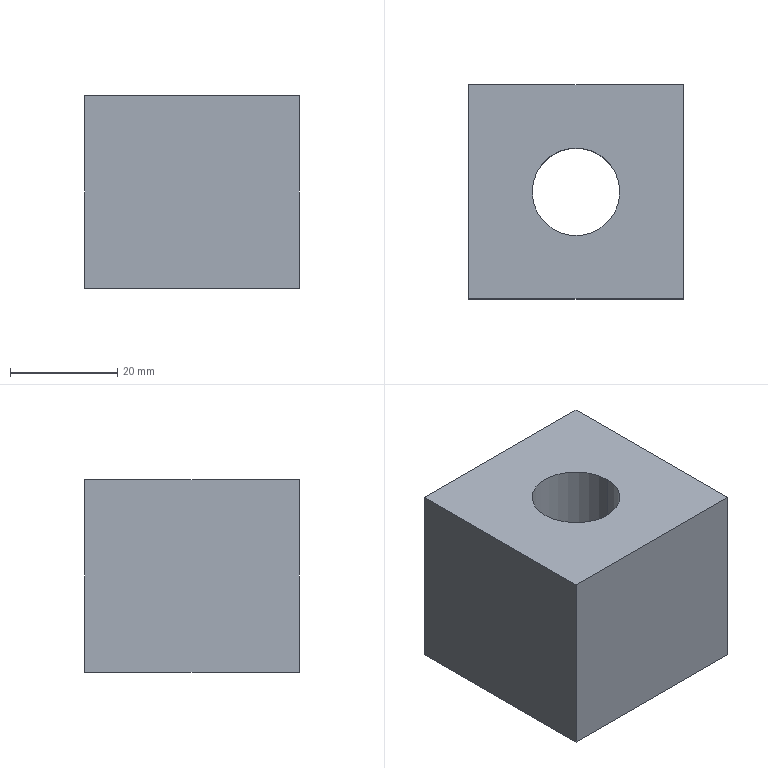Part | SolidWorks | features Extrusion 1, ICE 1 | 1 solid | 8 faces | box 40 x 40 x 36 mm | volume 49995 mm3 | plane 6 | cylinder 2 | commonest cylinder face diameters 16.4 x2
STEP:
#1=CARTESIAN_POINT('',(-8.2,0.,-18.));
#2=VERTEX_POINT('',#1);
#3=CARTESIAN_POINT('',(8.2,0.,-18.));
#4=VERTEX_POINT('',#3);
#5=CARTESIAN_POINT('',(0.,0.,-18.));
#6=DIRECTION('',(0.,0.,1.));
#7=DIRECTION('',(1.,0.,0.));
#8=AXIS2_PLACEMENT_3D('',#5,#6,#7);
#9=CIRCLE('',#8,8.2);
#10=EDGE_CURVE('',#2,#4,#9,.T.);
#11=ORIENTED_EDGE('',*,*,#10,.F.);
#12=CARTESIAN_POINT('',(-8.2,0.,18.));
#13=VERTEX_POINT('',#12);
#14=CARTESIAN_POINT('',(-8.2,0.,-30.));
#15=DIRECTION('',(0.,0.,1.));
#16=VECTOR('',#15,1000.);
#17=LINE('',#14,#16);
#18=EDGE_CURVE('',#2,#13,#17,.T.);
#19=ORIENTED_EDGE('',*,*,#18,.T.);
#20=CARTESIAN_POINT('',(8.2,0.,18.));
#21=VERTEX_POINT('',#20);
#22=CARTESIAN_POINT('',(0.,0.,18.));
#23=DIRECTION('',(0.,0.,1.));
#24=DIRECTION('',(1.,0.,0.));
#25=AXIS2_PLACEMENT_3D('',#22,#23,#24);
#26=CIRCLE('',#25,8.2);
#27=EDGE_CURVE('',#13,#21,#26,.T.);
#28=ORIENTED_EDGE('',*,*,#27,.T.);
#29=CARTESIAN_POINT('',(8.2,0.,-30.));
#30=DIRECTION('',(0.,0.,1.));
#31=VECTOR('',#30,1000.);
#32=LINE('',#29,#31);
#33=EDGE_CURVE('',#4,#21,#32,.T.);
#34=ORIENTED_EDGE('',*,*,#33,.F.);
#35=EDGE_LOOP('',(#11,#19,#28,#34));
#36=FACE_OUTER_BOUND('',#35,.T.);
#37=CARTESIAN_POINT('',(0.,0.,-30.));
#38=DIRECTION('',(0.,0.,1.));
#39=DIRECTION('',(1.,0.,0.));
#40=AXIS2_PLACEMENT_3D('',#37,#38,#39);
#41=CYLINDRICAL_SURFACE('',#40,8.2);
#42=ADVANCED_FACE('',(#36),#41,.F.);
#43=CARTESIAN_POINT('',(-20.,20.,18.));
#44=VERTEX_POINT('',#43);
#45=CARTESIAN_POINT('',(-20.,-20.,18.));
#46=VERTEX_POINT('',#45);
#47=CARTESIAN_POINT('',(-20.,20.,18.));
#48=DIRECTION('',(0.,-1.,0.));
#49=VECTOR('',#48,1000.);
#50=LINE('',#47,#49);
#51=EDGE_CURVE('',#44,#46,#50,.T.);
#52=ORIENTED_EDGE('',*,*,#51,.F.);
#53=CARTESIAN_POINT('',(-20.,20.,-18.));
#54=VERTEX_POINT('',#53);
#55=CARTESIAN_POINT('',(-20.,20.,-18.));
#56=DIRECTION('',(0.,0.,1.));
#57=VECTOR('',#56,1000.);
#58=LINE('',#55,#57);
#59=EDGE_CURVE('',#54,#44,#58,.T.);
#60=ORIENTED_EDGE('',*,*,#59,.F.);
#61=CARTESIAN_POINT('',(-20.,-20.,-18.));
#62=VERTEX_POINT('',#61);
#63=CARTESIAN_POINT('',(-20.,20.,-18.));
#64=DIRECTION('',(0.,-1.,0.));
#65=VECTOR('',#64,1000.);
#66=LINE('',#63,#65);
#67=EDGE_CURVE('',#54,#62,#66,.T.);
#68=ORIENTED_EDGE('',*,*,#67,.T.);
#69=CARTESIAN_POINT('',(-20.,-20.,-18.));
#70=DIRECTION('',(0.,0.,1.));
#71=VECTOR('',#70,1000.);
#72=LINE('',#69,#71);
#73=EDGE_CURVE('',#62,#46,#72,.T.);
#74=ORIENTED_EDGE('',*,*,#73,.T.);
#75=EDGE_LOOP('',(#52,#60,#68,#74));
#76=FACE_OUTER_BOUND('',#75,.T.);
#77=CARTESIAN_POINT('',(-20.,20.,-18.));
#78=DIRECTION('',(-1.,0.,0.));
#79=DIRECTION('',(0.,0.,1.));
#80=AXIS2_PLACEMENT_3D('',#77,#78,#79);
#81=PLANE('',#80);
#82=ADVANCED_FACE('',(#76),#81,.T.);
#83=CARTESIAN_POINT('',(20.,20.,18.));
#84=VERTEX_POINT('',#83);
#85=CARTESIAN_POINT('',(20.,20.,18.));
#86=DIRECTION('',(-1.,0.,0.));
#87=VECTOR('',#86,1000.);
#88=LINE('',#85,#87);
#89=EDGE_CURVE('',#84,#44,#88,.T.);
#90=ORIENTED_EDGE('',*,*,#89,.F.);
#91=CARTESIAN_POINT('',(20.,20.,-18.));
#92=VERTEX_POINT('',#91);
#93=CARTESIAN_POINT('',(20.,20.,-18.));
#94=DIRECTION('',(0.,0.,1.));
#95=VECTOR('',#94,1000.);
#96=LINE('',#93,#95);
#97=EDGE_CURVE('',#92,#84,#96,.T.);
#98=ORIENTED_EDGE('',*,*,#97,.F.);
#99=CARTESIAN_POINT('',(20.,20.,-18.));
#100=DIRECTION('',(-1.,0.,0.));
#101=VECTOR('',#100,1000.);
#102=LINE('',#99,#101);
#103=EDGE_CURVE('',#92,#54,#102,.T.);
#104=ORIENTED_EDGE('',*,*,#103,.T.);
#105=ORIENTED_EDGE('',*,*,#59,.T.);
#106=EDGE_LOOP('',(#90,#98,#104,#105));
#107=FACE_OUTER_BOUND('',#106,.T.);
#108=CARTESIAN_POINT('',(20.,20.,-18.));
#109=DIRECTION('',(0.,1.,0.));
#110=DIRECTION('',(0.,0.,1.));
#111=AXIS2_PLACEMENT_3D('',#108,#109,#110);
#112=PLANE('',#111);
#113=ADVANCED_FACE('',(#107),#112,.T.);
#114=CARTESIAN_POINT('',(20.,-20.,18.));
#115=VERTEX_POINT('',#114);
#116=CARTESIAN_POINT('',(20.,-20.,18.));
#117=DIRECTION('',(0.,1.,0.));
#118=VECTOR('',#117,1000.);
#119=LINE('',#116,#118);
#120=EDGE_CURVE('',#115,#84,#119,.T.);
#121=ORIENTED_EDGE('',*,*,#120,.F.);
#122=CARTESIAN_POINT('',(20.,-20.,-18.));
#123=VERTEX_POINT('',#122);
#124=CARTESIAN_POINT('',(20.,-20.,-18.));
#125=DIRECTION('',(0.,0.,1.));
#126=VECTOR('',#125,1000.);
#127=LINE('',#124,#126);
#128=EDGE_CURVE('',#123,#115,#127,.T.);
#129=ORIENTED_EDGE('',*,*,#128,.F.);
#130=CARTESIAN_POINT('',(20.,-20.,-18.));
#131=DIRECTION('',(0.,1.,0.));
#132=VECTOR('',#131,1000.);
#133=LINE('',#130,#132);
#134=EDGE_CURVE('',#123,#92,#133,.T.);
#135=ORIENTED_EDGE('',*,*,#134,.T.);
#136=ORIENTED_EDGE('',*,*,#97,.T.);
#137=EDGE_LOOP('',(#121,#129,#135,#136));
#138=FACE_OUTER_BOUND('',#137,.T.);
#139=CARTESIAN_POINT('',(20.,-20.,-18.));
#140=DIRECTION('',(1.,0.,0.));
#141=DIRECTION('',(0.,0.,-1.));
#142=AXIS2_PLACEMENT_3D('',#139,#140,#141);
#143=PLANE('',#142);
#144=ADVANCED_FACE('',(#138),#143,.T.);
#145=CARTESIAN_POINT('',(-20.,-20.,18.));
#146=DIRECTION('',(1.,0.,0.));
#147=VECTOR('',#146,1000.);
#148=LINE('',#145,#147);
#149=EDGE_CURVE('',#46,#115,#148,.T.);
#150=ORIENTED_EDGE('',*,*,#149,.F.);
#151=ORIENTED_EDGE('',*,*,#73,.F.);
#152=CARTESIAN_POINT('',(-20.,-20.,-18.));
#153=DIRECTION('',(1.,0.,0.));
#154=VECTOR('',#153,1000.);
#155=LINE('',#152,#154);
#156=EDGE_CURVE('',#62,#123,#155,.T.);
#157=ORIENTED_EDGE('',*,*,#156,.T.);
#158=ORIENTED_EDGE('',*,*,#128,.T.);
#159=EDGE_LOOP('',(#150,#151,#157,#158));
#160=FACE_OUTER_BOUND('',#159,.T.);
#161=CARTESIAN_POINT('',(-20.,-20.,-18.));
#162=DIRECTION('',(0.,-1.,0.));
#163=DIRECTION('',(0.,0.,-1.));
#164=AXIS2_PLACEMENT_3D('',#161,#162,#163);
#165=PLANE('',#164);
#166=ADVANCED_FACE('',(#160),#165,.T.);
#167=CARTESIAN_POINT('',(0.,0.,-18.));
#168=DIRECTION('',(0.,0.,1.));
#169=DIRECTION('',(1.,0.,0.));
#170=AXIS2_PLACEMENT_3D('',#167,#168,#169);
#171=CIRCLE('',#170,8.2);
#172=EDGE_CURVE('',#4,#2,#171,.T.);
#173=ORIENTED_EDGE('',*,*,#172,.T.);
#174=ORIENTED_EDGE('',*,*,#10,.T.);
#175=EDGE_LOOP('',(#173,#174));
#176=FACE_BOUND('',#175,.T.);
#177=ORIENTED_EDGE('',*,*,#67,.F.);
#178=ORIENTED_EDGE('',*,*,#103,.F.);
#179=ORIENTED_EDGE('',*,*,#134,.F.);
#180=ORIENTED_EDGE('',*,*,#156,.F.);
#181=EDGE_LOOP('',(#177,#178,#179,#180));
#182=FACE_OUTER_BOUND('',#181,.T.);
#183=CARTESIAN_POINT('',(0.,0.,-18.));
#184=DIRECTION('',(0.,0.,1.));
#185=DIRECTION('',(1.,0.,0.));
#186=AXIS2_PLACEMENT_3D('',#183,#184,#185);
#187=PLANE('',#186);
#188=ADVANCED_FACE('',(#176,#182),#187,.F.);
#189=CARTESIAN_POINT('',(0.,0.,18.));
#190=DIRECTION('',(0.,0.,1.));
#191=DIRECTION('',(1.,0.,0.));
#192=AXIS2_PLACEMENT_3D('',#189,#190,#191);
#193=CIRCLE('',#192,8.2);
#194=EDGE_CURVE('',#21,#13,#193,.T.);
#195=ORIENTED_EDGE('',*,*,#194,.F.);
#196=ORIENTED_EDGE('',*,*,#27,.F.);
#197=EDGE_LOOP('',(#195,#196));
#198=FACE_BOUND('',#197,.T.);
#199=ORIENTED_EDGE('',*,*,#51,.T.);
#200=ORIENTED_EDGE('',*,*,#149,.T.);
#201=ORIENTED_EDGE('',*,*,#120,.T.);
#202=ORIENTED_EDGE('',*,*,#89,.T.);
#203=EDGE_LOOP('',(#199,#200,#201,#202));
#204=FACE_OUTER_BOUND('',#203,.T.);
#205=CARTESIAN_POINT('',(0.,0.,18.));
#206=DIRECTION('',(0.,0.,1.));
#207=DIRECTION('',(1.,0.,0.));
#208=AXIS2_PLACEMENT_3D('',#205,#206,#207);
#209=PLANE('',#208);
#210=ADVANCED_FACE('',(#198,#204),#209,.T.);
#211=ORIENTED_EDGE('',*,*,#18,.F.);
#212=ORIENTED_EDGE('',*,*,#172,.F.);
#213=ORIENTED_EDGE('',*,*,#33,.T.);
#214=ORIENTED_EDGE('',*,*,#194,.T.);
#215=EDGE_LOOP('',(#211,#212,#213,#214));
#216=FACE_OUTER_BOUND('',#215,.T.);
#217=CARTESIAN_POINT('',(0.,0.,-30.));
#218=DIRECTION('',(0.,0.,1.));
#219=DIRECTION('',(1.,0.,0.));
#220=AXIS2_PLACEMENT_3D('',#217,#218,#219);
#221=CYLINDRICAL_SURFACE('',#220,8.2);
#222=ADVANCED_FACE('',(#216),#221,.F.);
#223=CLOSED_SHELL('',(#42,#82,#113,#144,#166,#188,#210,#222));
#224=MANIFOLD_SOLID_BREP('',#223);
#225=CARTESIAN_POINT('',(0.,0.,0.));
#226=DIRECTION('',(0.,0.,1.));
#227=DIRECTION('',(1.,0.,0.));
#228=AXIS2_PLACEMENT_3D('',#225,#226,#227);
#229=(LENGTH_UNIT()NAMED_UNIT(*)SI_UNIT(.MILLI.,.METRE.));
#230=UNCERTAINTY_MEASURE_WITH_UNIT(LENGTH_MEASURE(0.00001),#229,'','');
#231=(NAMED_UNIT(*)PLANE_ANGLE_UNIT()SI_UNIT($,.RADIAN.));
#232=(NAMED_UNIT(*)SI_UNIT($,.STERADIAN.)SOLID_ANGLE_UNIT());
#233=(GEOMETRIC_REPRESENTATION_CONTEXT(3)GLOBAL_UNCERTAINTY_ASSIGNED_CONTEXT((#230))GLOBAL_UNIT_ASSIGNED_CONTEXT((#229,#231,#232))REPRESENTATION_CONTEXT('',''));
#234=ADVANCED_BREP_SHAPE_REPRESENTATION('',(#224,#228),#233);